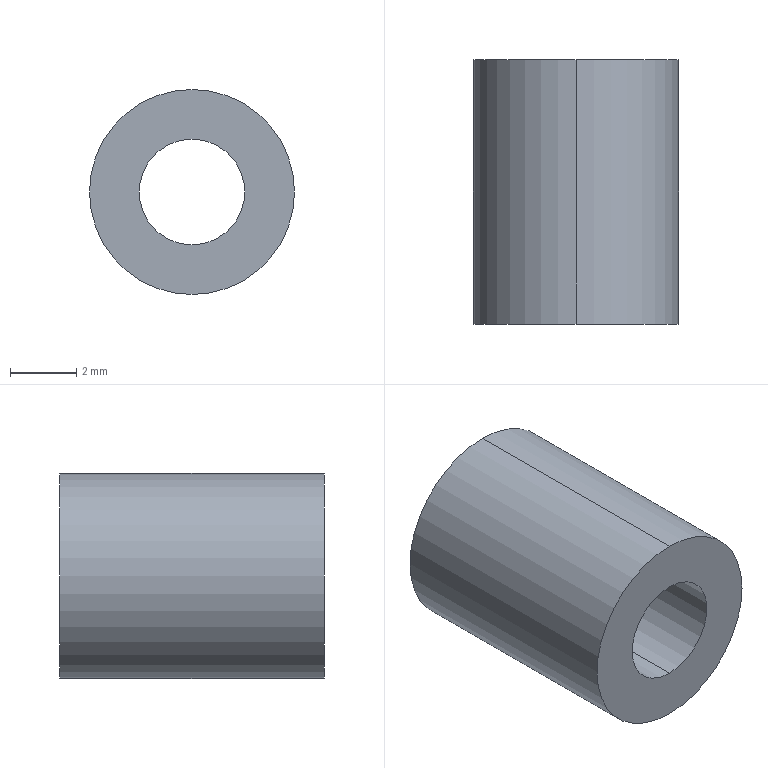Part | SolidWorks | features Extrusion 1 | 1 solid | 6 faces | box 6.2 x 8 x 6.2 mm | volume 177.186 mm3 | cylinder 4 | plane 2 | commonest cylinder face diameters 3.2 x2 6.2 x2
STEP:
#1=CARTESIAN_POINT('',(0.,8.,-1.6));
#2=VERTEX_POINT('',#1);
#3=CARTESIAN_POINT('',(0.,8.,1.6));
#4=VERTEX_POINT('',#3);
#5=CARTESIAN_POINT('',(0.,8.,0.));
#6=DIRECTION('',(0.,1.,0.));
#7=DIRECTION('',(0.,0.,1.));
#8=AXIS2_PLACEMENT_3D('',#5,#6,#7);
#9=CIRCLE('',#8,1.6);
#10=EDGE_CURVE('',#2,#4,#9,.T.);
#11=ORIENTED_EDGE('',*,*,#10,.T.);
#12=CARTESIAN_POINT('',(0.,0.,1.6));
#13=VERTEX_POINT('',#12);
#14=CARTESIAN_POINT('',(0.,8.,1.6));
#15=DIRECTION('',(0.,-1.,0.));
#16=VECTOR('',#15,1000.);
#17=LINE('',#14,#16);
#18=EDGE_CURVE('',#4,#13,#17,.T.);
#19=ORIENTED_EDGE('',*,*,#18,.T.);
#20=CARTESIAN_POINT('',(0.,0.,-1.6));
#21=VERTEX_POINT('',#20);
#22=CARTESIAN_POINT('',(0.,0.,0.));
#23=DIRECTION('',(0.,1.,0.));
#24=DIRECTION('',(0.,0.,1.));
#25=AXIS2_PLACEMENT_3D('',#22,#23,#24);
#26=CIRCLE('',#25,1.6);
#27=EDGE_CURVE('',#21,#13,#26,.T.);
#28=ORIENTED_EDGE('',*,*,#27,.F.);
#29=CARTESIAN_POINT('',(0.,8.,-1.6));
#30=DIRECTION('',(0.,-1.,0.));
#31=VECTOR('',#30,1000.);
#32=LINE('',#29,#31);
#33=EDGE_CURVE('',#2,#21,#32,.T.);
#34=ORIENTED_EDGE('',*,*,#33,.F.);
#35=EDGE_LOOP('',(#11,#19,#28,#34));
#36=FACE_OUTER_BOUND('',#35,.T.);
#37=CARTESIAN_POINT('',(0.,8.,0.));
#38=DIRECTION('',(0.,-1.,0.));
#39=DIRECTION('',(0.,0.,-1.));
#40=AXIS2_PLACEMENT_3D('',#37,#38,#39);
#41=CYLINDRICAL_SURFACE('',#40,1.6);
#42=ADVANCED_FACE('',(#36),#41,.F.);
#43=CARTESIAN_POINT('',(0.,8.,3.1));
#44=VERTEX_POINT('',#43);
#45=CARTESIAN_POINT('',(0.,8.,-3.1));
#46=VERTEX_POINT('',#45);
#47=CARTESIAN_POINT('',(0.,8.,0.));
#48=DIRECTION('',(0.,1.,0.));
#49=DIRECTION('',(0.,0.,1.));
#50=AXIS2_PLACEMENT_3D('',#47,#48,#49);
#51=CIRCLE('',#50,3.1);
#52=EDGE_CURVE('',#44,#46,#51,.T.);
#53=ORIENTED_EDGE('',*,*,#52,.F.);
#54=CARTESIAN_POINT('',(0.,0.,3.1));
#55=VERTEX_POINT('',#54);
#56=CARTESIAN_POINT('',(0.,8.,3.1));
#57=DIRECTION('',(0.,-1.,0.));
#58=VECTOR('',#57,1000.);
#59=LINE('',#56,#58);
#60=EDGE_CURVE('',#44,#55,#59,.T.);
#61=ORIENTED_EDGE('',*,*,#60,.T.);
#62=CARTESIAN_POINT('',(0.,0.,-3.1));
#63=VERTEX_POINT('',#62);
#64=CARTESIAN_POINT('',(0.,0.,0.));
#65=DIRECTION('',(0.,1.,0.));
#66=DIRECTION('',(0.,0.,1.));
#67=AXIS2_PLACEMENT_3D('',#64,#65,#66);
#68=CIRCLE('',#67,3.1);
#69=EDGE_CURVE('',#55,#63,#68,.T.);
#70=ORIENTED_EDGE('',*,*,#69,.T.);
#71=CARTESIAN_POINT('',(0.,8.,-3.1));
#72=DIRECTION('',(0.,-1.,0.));
#73=VECTOR('',#72,1000.);
#74=LINE('',#71,#73);
#75=EDGE_CURVE('',#46,#63,#74,.T.);
#76=ORIENTED_EDGE('',*,*,#75,.F.);
#77=EDGE_LOOP('',(#53,#61,#70,#76));
#78=FACE_OUTER_BOUND('',#77,.T.);
#79=CARTESIAN_POINT('',(0.,8.,0.));
#80=DIRECTION('',(0.,-1.,0.));
#81=DIRECTION('',(0.,0.,-1.));
#82=AXIS2_PLACEMENT_3D('',#79,#80,#81);
#83=CYLINDRICAL_SURFACE('',#82,3.1);
#84=ADVANCED_FACE('',(#78),#83,.T.);
#85=CARTESIAN_POINT('',(0.,8.,0.));
#86=DIRECTION('',(0.,1.,0.));
#87=DIRECTION('',(0.,0.,1.));
#88=AXIS2_PLACEMENT_3D('',#85,#86,#87);
#89=CIRCLE('',#88,3.1);
#90=EDGE_CURVE('',#46,#44,#89,.T.);
#91=ORIENTED_EDGE('',*,*,#90,.T.);
#92=ORIENTED_EDGE('',*,*,#52,.T.);
#93=EDGE_LOOP('',(#91,#92));
#94=FACE_OUTER_BOUND('',#93,.T.);
#95=ORIENTED_EDGE('',*,*,#10,.F.);
#96=CARTESIAN_POINT('',(0.,8.,0.));
#97=DIRECTION('',(0.,1.,0.));
#98=DIRECTION('',(0.,0.,1.));
#99=AXIS2_PLACEMENT_3D('',#96,#97,#98);
#100=CIRCLE('',#99,1.6);
#101=EDGE_CURVE('',#4,#2,#100,.T.);
#102=ORIENTED_EDGE('',*,*,#101,.F.);
#103=EDGE_LOOP('',(#95,#102));
#104=FACE_BOUND('',#103,.T.);
#105=CARTESIAN_POINT('',(0.,8.,0.));
#106=DIRECTION('',(0.,1.,0.));
#107=DIRECTION('',(0.,0.,1.));
#108=AXIS2_PLACEMENT_3D('',#105,#106,#107);
#109=PLANE('',#108);
#110=ADVANCED_FACE('',(#94,#104),#109,.T.);
#111=CARTESIAN_POINT('',(0.,0.,0.));
#112=DIRECTION('',(0.,1.,0.));
#113=DIRECTION('',(0.,0.,1.));
#114=AXIS2_PLACEMENT_3D('',#111,#112,#113);
#115=CIRCLE('',#114,3.1);
#116=EDGE_CURVE('',#63,#55,#115,.T.);
#117=ORIENTED_EDGE('',*,*,#116,.F.);
#118=ORIENTED_EDGE('',*,*,#69,.F.);
#119=EDGE_LOOP('',(#117,#118));
#120=FACE_OUTER_BOUND('',#119,.T.);
#121=ORIENTED_EDGE('',*,*,#27,.T.);
#122=CARTESIAN_POINT('',(0.,0.,0.));
#123=DIRECTION('',(0.,1.,0.));
#124=DIRECTION('',(0.,0.,1.));
#125=AXIS2_PLACEMENT_3D('',#122,#123,#124);
#126=CIRCLE('',#125,1.6);
#127=EDGE_CURVE('',#13,#21,#126,.T.);
#128=ORIENTED_EDGE('',*,*,#127,.T.);
#129=EDGE_LOOP('',(#121,#128));
#130=FACE_BOUND('',#129,.T.);
#131=CARTESIAN_POINT('',(0.,0.,0.));
#132=DIRECTION('',(0.,1.,0.));
#133=DIRECTION('',(0.,0.,1.));
#134=AXIS2_PLACEMENT_3D('',#131,#132,#133);
#135=PLANE('',#134);
#136=ADVANCED_FACE('',(#120,#130),#135,.F.);
#137=ORIENTED_EDGE('',*,*,#60,.F.);
#138=ORIENTED_EDGE('',*,*,#90,.F.);
#139=ORIENTED_EDGE('',*,*,#75,.T.);
#140=ORIENTED_EDGE('',*,*,#116,.T.);
#141=EDGE_LOOP('',(#137,#138,#139,#140));
#142=FACE_OUTER_BOUND('',#141,.T.);
#143=CARTESIAN_POINT('',(0.,8.,0.));
#144=DIRECTION('',(0.,-1.,0.));
#145=DIRECTION('',(0.,0.,-1.));
#146=AXIS2_PLACEMENT_3D('',#143,#144,#145);
#147=CYLINDRICAL_SURFACE('',#146,3.1);
#148=ADVANCED_FACE('',(#142),#147,.T.);
#149=ORIENTED_EDGE('',*,*,#18,.F.);
#150=ORIENTED_EDGE('',*,*,#101,.T.);
#151=ORIENTED_EDGE('',*,*,#33,.T.);
#152=ORIENTED_EDGE('',*,*,#127,.F.);
#153=EDGE_LOOP('',(#149,#150,#151,#152));
#154=FACE_OUTER_BOUND('',#153,.T.);
#155=CARTESIAN_POINT('',(0.,8.,0.));
#156=DIRECTION('',(0.,-1.,0.));
#157=DIRECTION('',(0.,0.,-1.));
#158=AXIS2_PLACEMENT_3D('',#155,#156,#157);
#159=CYLINDRICAL_SURFACE('',#158,1.6);
#160=ADVANCED_FACE('',(#154),#159,.F.);
#161=CLOSED_SHELL('',(#42,#84,#110,#136,#148,#160));
#162=MANIFOLD_SOLID_BREP('',#161);
#163=CARTESIAN_POINT('',(0.,0.,0.));
#164=DIRECTION('',(0.,0.,1.));
#165=DIRECTION('',(1.,0.,0.));
#166=AXIS2_PLACEMENT_3D('',#163,#164,#165);
#167=(LENGTH_UNIT()NAMED_UNIT(*)SI_UNIT(.MILLI.,.METRE.));
#168=UNCERTAINTY_MEASURE_WITH_UNIT(LENGTH_MEASURE(0.00001),#167,'','');
#169=(NAMED_UNIT(*)PLANE_ANGLE_UNIT()SI_UNIT($,.RADIAN.));
#170=(NAMED_UNIT(*)SI_UNIT($,.STERADIAN.)SOLID_ANGLE_UNIT());
#171=(GEOMETRIC_REPRESENTATION_CONTEXT(3)GLOBAL_UNCERTAINTY_ASSIGNED_CONTEXT((#168))GLOBAL_UNIT_ASSIGNED_CONTEXT((#167,#169,#170))REPRESENTATION_CONTEXT('',''));
#172=ADVANCED_BREP_SHAPE_REPRESENTATION('',(#162,#166),#171);